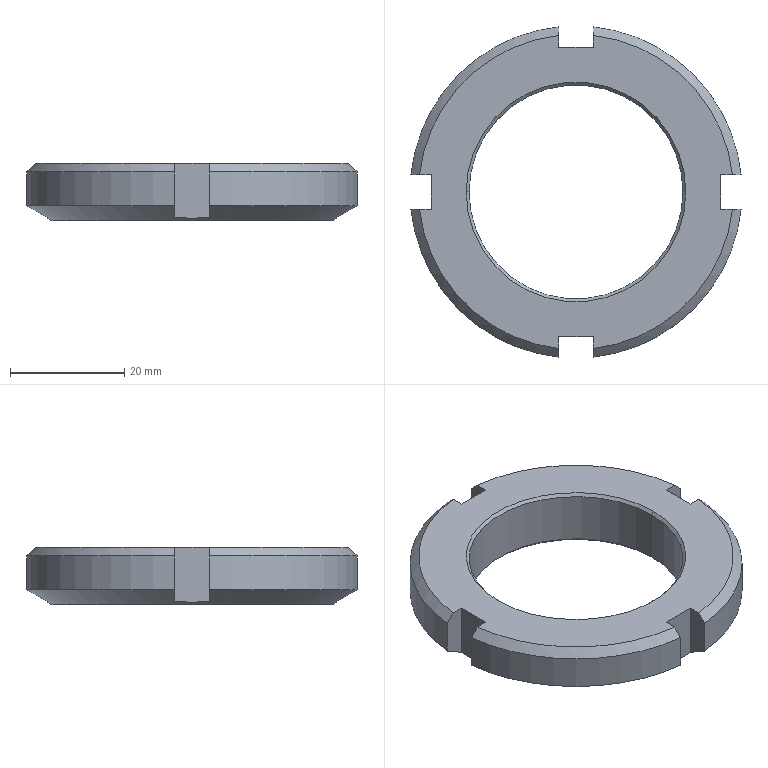Part | SolidWorks | features Chamfer 3, CirPattern 1, Cut 1, Extrusion 1 | 1 solid | 30 faces | box 57.689 x 57.689 x 10 mm | volume 13482 mm3 | plane 14 | cone 10 | cylinder 6 | commonest cylinder face diameters 58 x4 37.376 x2
STEP:
#1=CARTESIAN_POINT('',(-18.688,0.,9.5));
#2=VERTEX_POINT('',#1);
#3=CARTESIAN_POINT('',(18.688,0.,9.5));
#4=VERTEX_POINT('',#3);
#5=CARTESIAN_POINT('',(0.,0.,9.5));
#6=DIRECTION('',(0.,0.,1.));
#7=DIRECTION('',(1.,0.,0.));
#8=AXIS2_PLACEMENT_3D('',#5,#6,#7);
#9=CIRCLE('',#8,18.688);
#10=EDGE_CURVE('',#2,#4,#9,.T.);
#11=ORIENTED_EDGE('',*,*,#10,.F.);
#12=CARTESIAN_POINT('',(-19.188,0.,10.));
#13=VERTEX_POINT('',#12);
#14=CARTESIAN_POINT('',(-18.688,0.,9.5));
#15=DIRECTION('',(-0.7071,0.,0.7071));
#16=VECTOR('',#15,1000.);
#17=LINE('',#14,#16);
#18=EDGE_CURVE('',#2,#13,#17,.T.);
#19=ORIENTED_EDGE('',*,*,#18,.T.);
#20=CARTESIAN_POINT('',(19.188,0.,10.));
#21=VERTEX_POINT('',#20);
#22=CARTESIAN_POINT('',(0.,0.,10.));
#23=DIRECTION('',(0.,0.,-1.));
#24=DIRECTION('',(1.,0.,0.));
#25=AXIS2_PLACEMENT_3D('',#22,#23,#24);
#26=CIRCLE('',#25,19.188);
#27=EDGE_CURVE('',#21,#13,#26,.T.);
#28=ORIENTED_EDGE('',*,*,#27,.F.);
#29=CARTESIAN_POINT('',(18.688,0.,9.5));
#30=DIRECTION('',(0.7071,0.,0.7071));
#31=VECTOR('',#30,1000.);
#32=LINE('',#29,#31);
#33=EDGE_CURVE('',#4,#21,#32,.T.);
#34=ORIENTED_EDGE('',*,*,#33,.F.);
#35=EDGE_LOOP('',(#11,#19,#28,#34));
#36=FACE_OUTER_BOUND('',#35,.T.);
#37=CARTESIAN_POINT('',(0.,0.,9.5));
#38=DIRECTION('',(0.,0.,1.));
#39=DIRECTION('',(1.,0.,0.));
#40=AXIS2_PLACEMENT_3D('',#37,#38,#39);
#41=CONICAL_SURFACE('',#40,18.688,0.7854);
#42=ADVANCED_FACE('',(#36),#41,.F.);
#43=CARTESIAN_POINT('',(18.688,0.,0.5));
#44=VERTEX_POINT('',#43);
#45=CARTESIAN_POINT('',(-18.688,0.,0.5));
#46=VERTEX_POINT('',#45);
#47=CARTESIAN_POINT('',(0.,0.,0.5));
#48=DIRECTION('',(0.,0.,-1.));
#49=DIRECTION('',(1.,0.,0.));
#50=AXIS2_PLACEMENT_3D('',#47,#48,#49);
#51=CIRCLE('',#50,18.688);
#52=EDGE_CURVE('',#44,#46,#51,.T.);
#53=ORIENTED_EDGE('',*,*,#52,.F.);
#54=CARTESIAN_POINT('',(19.188,0.,0.));
#55=VERTEX_POINT('',#54);
#56=CARTESIAN_POINT('',(19.188,0.,0.));
#57=DIRECTION('',(0.7071,0.,-0.7071));
#58=VECTOR('',#57,1000.);
#59=LINE('',#56,#58);
#60=EDGE_CURVE('',#44,#55,#59,.T.);
#61=ORIENTED_EDGE('',*,*,#60,.T.);
#62=CARTESIAN_POINT('',(-19.188,0.,0.));
#63=VERTEX_POINT('',#62);
#64=CARTESIAN_POINT('',(0.,0.,0.));
#65=DIRECTION('',(0.,0.,1.));
#66=DIRECTION('',(1.,0.,0.));
#67=AXIS2_PLACEMENT_3D('',#64,#65,#66);
#68=CIRCLE('',#67,19.188);
#69=EDGE_CURVE('',#63,#55,#68,.T.);
#70=ORIENTED_EDGE('',*,*,#69,.F.);
#71=CARTESIAN_POINT('',(-19.188,0.,0.));
#72=DIRECTION('',(-0.7071,0.,-0.7071));
#73=VECTOR('',#72,1000.);
#74=LINE('',#71,#73);
#75=EDGE_CURVE('',#46,#63,#74,.T.);
#76=ORIENTED_EDGE('',*,*,#75,.F.);
#77=EDGE_LOOP('',(#53,#61,#70,#76));
#78=FACE_OUTER_BOUND('',#77,.T.);
#79=CARTESIAN_POINT('',(0.,0.,0.));
#80=DIRECTION('',(0.,0.,-1.));
#81=DIRECTION('',(-1.,0.,0.));
#82=AXIS2_PLACEMENT_3D('',#79,#80,#81);
#83=CONICAL_SURFACE('',#82,19.188,0.7854);
#84=ADVANCED_FACE('',(#78),#83,.F.);
#85=CARTESIAN_POINT('',(-24.5,0.,0.));
#86=VERTEX_POINT('',#85);
#87=CARTESIAN_POINT('',(24.5,0.,0.));
#88=VERTEX_POINT('',#87);
#89=CARTESIAN_POINT('',(0.,0.,0.));
#90=DIRECTION('',(0.,0.,-1.));
#91=DIRECTION('',(1.,0.,0.));
#92=AXIS2_PLACEMENT_3D('',#89,#90,#91);
#93=CIRCLE('',#92,24.5);
#94=EDGE_CURVE('',#86,#88,#93,.T.);
#95=ORIENTED_EDGE('',*,*,#94,.F.);
#96=CARTESIAN_POINT('',(-25.244,0.,0.4298));
#97=VERTEX_POINT('',#96);
#98=CARTESIAN_POINT('',(-29.,0.,2.598));
#99=DIRECTION('',(-0.866,0.,0.5));
#100=VECTOR('',#99,1000.);
#101=LINE('',#98,#100);
#102=EDGE_CURVE('',#86,#97,#101,.T.);
#103=ORIENTED_EDGE('',*,*,#102,.T.);
#104=CARTESIAN_POINT('',(-25.244,3.,0.5323));
#105=VERTEX_POINT('',#104);
#106=CARTESIAN_POINT('',(-25.244,3.,0.5323));
#107=CARTESIAN_POINT('',(-25.244,2.003,0.4644));
#108=CARTESIAN_POINT('',(-25.244,1.003,0.4298));
#109=CARTESIAN_POINT('',(-25.244,0.,0.4298));
#110=B_SPLINE_CURVE_WITH_KNOTS('',3,(#106,#107,#108,#109),.UNSPECIFIED.,.F.,.F.,(4,4),(0.007992,0.01099),.UNSPECIFIED.);
#111=EDGE_CURVE('',#105,#97,#110,.T.);
#112=ORIENTED_EDGE('',*,*,#111,.F.);
#113=CARTESIAN_POINT('',(-28.844,3.,2.598));
#114=VERTEX_POINT('',#113);
#115=CARTESIAN_POINT('',(-28.844,3.,2.598));
#116=CARTESIAN_POINT('',(-28.638,3.,2.48));
#117=CARTESIAN_POINT('',(-28.432,3.,2.361));
#118=CARTESIAN_POINT('',(-28.226,3.,2.243));
#119=CARTESIAN_POINT('',(-27.232,3.,1.672));
#120=CARTESIAN_POINT('',(-26.238,3.,1.102));
#121=CARTESIAN_POINT('',(-25.244,3.,0.5323));
#122=B_SPLINE_CURVE_WITH_KNOTS('',3,(#115,#116,#117,#118,#119,#120,#121),.UNSPECIFIED.,.F.,.F.,(4,3,4),(0.007772,0.008485,0.01192),.UNSPECIFIED.);
#123=EDGE_CURVE('',#114,#105,#122,.T.);
#124=ORIENTED_EDGE('',*,*,#123,.F.);
#125=CARTESIAN_POINT('',(-3.,28.844,2.598));
#126=VERTEX_POINT('',#125);
#127=CARTESIAN_POINT('',(0.,0.,2.598));
#128=DIRECTION('',(0.,0.,1.));
#129=DIRECTION('',(1.,0.,0.));
#130=AXIS2_PLACEMENT_3D('',#127,#128,#129);
#131=CIRCLE('',#130,29.);
#132=EDGE_CURVE('',#126,#114,#131,.T.);
#133=ORIENTED_EDGE('',*,*,#132,.F.);
#134=CARTESIAN_POINT('',(-3.,25.244,0.5323));
#135=VERTEX_POINT('',#134);
#136=CARTESIAN_POINT('',(-3.,25.244,0.5323));
#137=CARTESIAN_POINT('',(-3.,26.445,1.22));
#138=CARTESIAN_POINT('',(-3.,27.645,1.909));
#139=CARTESIAN_POINT('',(-3.,28.844,2.598));
#140=B_SPLINE_CURVE_WITH_KNOTS('',3,(#136,#137,#138,#139),.UNSPECIFIED.,.F.,.F.,(4,4),(0.008037,0.01219),.UNSPECIFIED.);
#141=EDGE_CURVE('',#135,#126,#140,.T.);
#142=ORIENTED_EDGE('',*,*,#141,.F.);
#143=CARTESIAN_POINT('',(3.,25.244,0.5323));
#144=VERTEX_POINT('',#143);
#145=CARTESIAN_POINT('',(3.,25.244,0.5323));
#146=CARTESIAN_POINT('',(2.006,25.244,0.4646));
#147=CARTESIAN_POINT('',(1.009,25.244,0.43));
#148=CARTESIAN_POINT('',(-0.9914,25.244,0.4296));
#149=CARTESIAN_POINT('',(-1.998,25.244,0.4641));
#150=CARTESIAN_POINT('',(-3.,25.244,0.5323));
#151=B_SPLINE_CURVE_WITH_KNOTS('',3,(#145,#146,#147,#148,#149,#150),.UNSPECIFIED.,.F.,.F.,(4,2,4),(0.007992,0.01098,0.01397),.UNSPECIFIED.);
#152=EDGE_CURVE('',#144,#135,#151,.T.);
#153=ORIENTED_EDGE('',*,*,#152,.F.);
#154=CARTESIAN_POINT('',(3.,28.844,2.598));
#155=VERTEX_POINT('',#154);
#156=CARTESIAN_POINT('',(3.,28.844,2.598));
#157=CARTESIAN_POINT('',(3.,27.645,1.909));
#158=CARTESIAN_POINT('',(3.,26.445,1.22));
#159=CARTESIAN_POINT('',(3.,25.244,0.5323));
#160=B_SPLINE_CURVE_WITH_KNOTS('',3,(#156,#157,#158,#159),.UNSPECIFIED.,.F.,.F.,(4,4),(0.004783,0.008934),.UNSPECIFIED.);
#161=EDGE_CURVE('',#155,#144,#160,.T.);
#162=ORIENTED_EDGE('',*,*,#161,.F.);
#163=CARTESIAN_POINT('',(28.844,3.,2.598));
#164=VERTEX_POINT('',#163);
#165=CARTESIAN_POINT('',(0.,0.,2.598));
#166=DIRECTION('',(0.,0.,1.));
#167=DIRECTION('',(1.,0.,0.));
#168=AXIS2_PLACEMENT_3D('',#165,#166,#167);
#169=CIRCLE('',#168,29.);
#170=EDGE_CURVE('',#164,#155,#169,.T.);
#171=ORIENTED_EDGE('',*,*,#170,.F.);
#172=CARTESIAN_POINT('',(25.244,3.,0.5323));
#173=VERTEX_POINT('',#172);
#174=CARTESIAN_POINT('',(25.244,3.,0.5323));
#175=CARTESIAN_POINT('',(26.445,3.,1.22));
#176=CARTESIAN_POINT('',(27.645,3.,1.909));
#177=CARTESIAN_POINT('',(28.844,3.,2.598));
#178=B_SPLINE_CURVE_WITH_KNOTS('',3,(#174,#175,#176,#177),.UNSPECIFIED.,.F.,.F.,(4,4),(0.008037,0.01219),.UNSPECIFIED.);
#179=EDGE_CURVE('',#173,#164,#178,.T.);
#180=ORIENTED_EDGE('',*,*,#179,.F.);
#181=CARTESIAN_POINT('',(25.244,0.,0.4298));
#182=VERTEX_POINT('',#181);
#183=CARTESIAN_POINT('',(25.244,0.,0.4298));
#184=CARTESIAN_POINT('',(25.244,1.003,0.4298));
#185=CARTESIAN_POINT('',(25.244,2.003,0.4644));
#186=CARTESIAN_POINT('',(25.244,3.,0.5323));
#187=B_SPLINE_CURVE_WITH_KNOTS('',3,(#183,#184,#185,#186),.UNSPECIFIED.,.F.,.F.,(4,4),(0.01545,0.01845),.UNSPECIFIED.);
#188=EDGE_CURVE('',#182,#173,#187,.T.);
#189=ORIENTED_EDGE('',*,*,#188,.F.);
#190=CARTESIAN_POINT('',(29.,0.,2.598));
#191=DIRECTION('',(0.866,0.,0.5));
#192=VECTOR('',#191,1000.);
#193=LINE('',#190,#192);
#194=EDGE_CURVE('',#88,#182,#193,.T.);
#195=ORIENTED_EDGE('',*,*,#194,.F.);
#196=EDGE_LOOP('',(#95,#103,#112,#124,#133,#142,#153,#162,#171,#180,#189,#195));
#197=FACE_OUTER_BOUND('',#196,.T.);
#198=CARTESIAN_POINT('',(0.,0.,2.598));
#199=DIRECTION('',(0.,0.,1.));
#200=DIRECTION('',(1.,0.,0.));
#201=AXIS2_PLACEMENT_3D('',#198,#199,#200);
#202=CONICAL_SURFACE('',#201,29.,1.047);
#203=ADVANCED_FACE('',(#197),#202,.T.);
#204=ORIENTED_EDGE('',*,*,#10,.T.);
#205=CARTESIAN_POINT('',(18.688,0.,10.));
#206=DIRECTION('',(0.,0.,-1.));
#207=VECTOR('',#206,1000.);
#208=LINE('',#205,#207);
#209=EDGE_CURVE('',#4,#44,#208,.T.);
#210=ORIENTED_EDGE('',*,*,#209,.T.);
#211=ORIENTED_EDGE('',*,*,#52,.T.);
#212=CARTESIAN_POINT('',(-18.688,0.,10.));
#213=DIRECTION('',(0.,0.,-1.));
#214=VECTOR('',#213,1000.);
#215=LINE('',#212,#214);
#216=EDGE_CURVE('',#2,#46,#215,.T.);
#217=ORIENTED_EDGE('',*,*,#216,.F.);
#218=EDGE_LOOP('',(#204,#210,#211,#217));
#219=FACE_OUTER_BOUND('',#218,.T.);
#220=CARTESIAN_POINT('',(0.,0.,10.));
#221=DIRECTION('',(0.,0.,-1.));
#222=DIRECTION('',(-1.,0.,0.));
#223=AXIS2_PLACEMENT_3D('',#220,#221,#222);
#224=CYLINDRICAL_SURFACE('',#223,18.688);
#225=ADVANCED_FACE('',(#219),#224,.F.);
#226=CARTESIAN_POINT('',(3.,28.844,8.5));
#227=VERTEX_POINT('',#226);
#228=CARTESIAN_POINT('',(28.844,3.,8.5));
#229=VERTEX_POINT('',#228);
#230=CARTESIAN_POINT('',(0.,0.,8.5));
#231=DIRECTION('',(0.,0.,-1.));
#232=DIRECTION('',(1.,0.,0.));
#233=AXIS2_PLACEMENT_3D('',#230,#231,#232);
#234=CIRCLE('',#233,29.);
#235=EDGE_CURVE('',#227,#229,#234,.T.);
#236=ORIENTED_EDGE('',*,*,#235,.T.);
#237=CARTESIAN_POINT('',(28.844,3.,0.));
#238=DIRECTION('',(0.,0.,1.));
#239=VECTOR('',#238,1000.);
#240=LINE('',#237,#239);
#241=EDGE_CURVE('',#164,#229,#240,.T.);
#242=ORIENTED_EDGE('',*,*,#241,.F.);
#243=ORIENTED_EDGE('',*,*,#170,.T.);
#244=CARTESIAN_POINT('',(3.,28.844,0.));
#245=DIRECTION('',(0.,0.,1.));
#246=VECTOR('',#245,1000.);
#247=LINE('',#244,#246);
#248=EDGE_CURVE('',#155,#227,#247,.T.);
#249=ORIENTED_EDGE('',*,*,#248,.T.);
#250=EDGE_LOOP('',(#236,#242,#243,#249));
#251=FACE_OUTER_BOUND('',#250,.T.);
#252=CARTESIAN_POINT('',(0.,0.,10.));
#253=DIRECTION('',(0.,0.,-1.));
#254=DIRECTION('',(-1.,0.,0.));
#255=AXIS2_PLACEMENT_3D('',#252,#253,#254);
#256=CYLINDRICAL_SURFACE('',#255,29.);
#257=ADVANCED_FACE('',(#251),#256,.T.);
#258=CARTESIAN_POINT('',(27.336,3.,10.));
#259=VERTEX_POINT('',#258);
#260=CARTESIAN_POINT('',(28.844,3.,8.5));
#261=CARTESIAN_POINT('',(28.431,3.,8.911));
#262=CARTESIAN_POINT('',(28.017,3.,9.323));
#263=CARTESIAN_POINT('',(27.603,3.,9.734));
#264=CARTESIAN_POINT('',(27.514,3.,9.823));
#265=CARTESIAN_POINT('',(27.425,3.,9.911));
#266=CARTESIAN_POINT('',(27.336,3.,10.));
#267=B_SPLINE_CURVE_WITH_KNOTS('',3,(#260,#261,#262,#263,#264,#265,#266),.UNSPECIFIED.,.F.,.F.,(4,3,4),(0.006071,0.007821,0.008198),.UNSPECIFIED.);
#268=EDGE_CURVE('',#229,#259,#267,.T.);
#269=ORIENTED_EDGE('',*,*,#268,.F.);
#270=ORIENTED_EDGE('',*,*,#235,.F.);
#271=CARTESIAN_POINT('',(3.,27.336,10.));
#272=VERTEX_POINT('',#271);
#273=CARTESIAN_POINT('',(3.,27.336,10.));
#274=CARTESIAN_POINT('',(3.,27.425,9.911));
#275=CARTESIAN_POINT('',(3.,27.514,9.823));
#276=CARTESIAN_POINT('',(3.,27.603,9.734));
#277=CARTESIAN_POINT('',(3.,28.017,9.323));
#278=CARTESIAN_POINT('',(3.,28.431,8.911));
#279=CARTESIAN_POINT('',(3.,28.844,8.5));
#280=B_SPLINE_CURVE_WITH_KNOTS('',3,(#273,#274,#275,#276,#277,#278,#279),.UNSPECIFIED.,.F.,.F.,(4,3,4),(0.007445,0.007821,0.009572),.UNSPECIFIED.);
#281=EDGE_CURVE('',#272,#227,#280,.T.);
#282=ORIENTED_EDGE('',*,*,#281,.F.);
#283=CARTESIAN_POINT('',(0.,0.,10.));
#284=DIRECTION('',(0.,0.,1.));
#285=DIRECTION('',(1.,0.,0.));
#286=AXIS2_PLACEMENT_3D('',#283,#284,#285);
#287=CIRCLE('',#286,27.5);
#288=EDGE_CURVE('',#259,#272,#287,.T.);
#289=ORIENTED_EDGE('',*,*,#288,.F.);
#290=EDGE_LOOP('',(#269,#270,#282,#289));
#291=FACE_OUTER_BOUND('',#290,.T.);
#292=CARTESIAN_POINT('',(0.,0.,10.));
#293=DIRECTION('',(0.,0.,-1.));
#294=DIRECTION('',(-1.,0.,0.));
#295=AXIS2_PLACEMENT_3D('',#292,#293,#294);
#296=CONICAL_SURFACE('',#295,27.5,0.7854);
#297=ADVANCED_FACE('',(#291),#296,.T.);
#298=CARTESIAN_POINT('',(-28.844,3.,8.5));
#299=VERTEX_POINT('',#298);
#300=CARTESIAN_POINT('',(-3.,28.844,8.5));
#301=VERTEX_POINT('',#300);
#302=CARTESIAN_POINT('',(0.,0.,8.5));
#303=DIRECTION('',(0.,0.,-1.));
#304=DIRECTION('',(1.,0.,0.));
#305=AXIS2_PLACEMENT_3D('',#302,#303,#304);
#306=CIRCLE('',#305,29.);
#307=EDGE_CURVE('',#299,#301,#306,.T.);
#308=ORIENTED_EDGE('',*,*,#307,.T.);
#309=CARTESIAN_POINT('',(-3.,28.844,0.));
#310=DIRECTION('',(0.,0.,1.));
#311=VECTOR('',#310,1000.);
#312=LINE('',#309,#311);
#313=EDGE_CURVE('',#126,#301,#312,.T.);
#314=ORIENTED_EDGE('',*,*,#313,.F.);
#315=ORIENTED_EDGE('',*,*,#132,.T.);
#316=CARTESIAN_POINT('',(-28.844,3.,0.));
#317=DIRECTION('',(0.,0.,1.));
#318=VECTOR('',#317,1000.);
#319=LINE('',#316,#318);
#320=EDGE_CURVE('',#114,#299,#319,.T.);
#321=ORIENTED_EDGE('',*,*,#320,.T.);
#322=EDGE_LOOP('',(#308,#314,#315,#321));
#323=FACE_OUTER_BOUND('',#322,.T.);
#324=CARTESIAN_POINT('',(0.,0.,10.));
#325=DIRECTION('',(0.,0.,-1.));
#326=DIRECTION('',(-1.,0.,0.));
#327=AXIS2_PLACEMENT_3D('',#324,#325,#326);
#328=CYLINDRICAL_SURFACE('',#327,29.);
#329=ADVANCED_FACE('',(#323),#328,.T.);
#330=CARTESIAN_POINT('',(-3.,27.336,10.));
#331=VERTEX_POINT('',#330);
#332=CARTESIAN_POINT('',(-3.,28.844,8.5));
#333=CARTESIAN_POINT('',(-3.,28.431,8.911));
#334=CARTESIAN_POINT('',(-3.,28.017,9.323));
#335=CARTESIAN_POINT('',(-3.,27.603,9.734));
#336=CARTESIAN_POINT('',(-3.,27.514,9.823));
#337=CARTESIAN_POINT('',(-3.,27.425,9.911));
#338=CARTESIAN_POINT('',(-3.,27.336,10.));
#339=B_SPLINE_CURVE_WITH_KNOTS('',3,(#332,#333,#334,#335,#336,#337,#338),.UNSPECIFIED.,.F.,.F.,(4,3,4),(0.006071,0.007821,0.008198),.UNSPECIFIED.);
#340=EDGE_CURVE('',#301,#331,#339,.T.);
#341=ORIENTED_EDGE('',*,*,#340,.F.);
#342=ORIENTED_EDGE('',*,*,#307,.F.);
#343=CARTESIAN_POINT('',(-27.336,3.,10.));
#344=VERTEX_POINT('',#343);
#345=CARTESIAN_POINT('',(-27.336,3.,10.));
#346=CARTESIAN_POINT('',(-27.701,3.,9.637));
#347=CARTESIAN_POINT('',(-28.066,3.,9.274));
#348=CARTESIAN_POINT('',(-28.431,3.,8.911));
#349=CARTESIAN_POINT('',(-28.569,3.,8.774));
#350=CARTESIAN_POINT('',(-28.707,3.,8.637));
#351=CARTESIAN_POINT('',(-28.844,3.,8.5));
#352=B_SPLINE_CURVE_WITH_KNOTS('',3,(#345,#346,#347,#348,#349,#350,#351),.UNSPECIFIED.,.F.,.F.,(4,3,4),(0.006278,0.007821,0.008405),.UNSPECIFIED.);
#353=EDGE_CURVE('',#344,#299,#352,.T.);
#354=ORIENTED_EDGE('',*,*,#353,.F.);
#355=CARTESIAN_POINT('',(0.,0.,10.));
#356=DIRECTION('',(0.,0.,1.));
#357=DIRECTION('',(1.,0.,0.));
#358=AXIS2_PLACEMENT_3D('',#355,#356,#357);
#359=CIRCLE('',#358,27.5);
#360=EDGE_CURVE('',#331,#344,#359,.T.);
#361=ORIENTED_EDGE('',*,*,#360,.F.);
#362=EDGE_LOOP('',(#341,#342,#354,#361));
#363=FACE_OUTER_BOUND('',#362,.T.);
#364=CARTESIAN_POINT('',(0.,0.,10.));
#365=DIRECTION('',(0.,0.,-1.));
#366=DIRECTION('',(-1.,0.,0.));
#367=AXIS2_PLACEMENT_3D('',#364,#365,#366);
#368=CONICAL_SURFACE('',#367,27.5,0.7854);
#369=ADVANCED_FACE('',(#363),#368,.T.);
#370=CARTESIAN_POINT('',(-3.,-28.844,8.5));
#371=VERTEX_POINT('',#370);
#372=CARTESIAN_POINT('',(-28.844,-3.,8.5));
#373=VERTEX_POINT('',#372);
#374=CARTESIAN_POINT('',(0.,0.,8.5));
#375=DIRECTION('',(0.,0.,-1.));
#376=DIRECTION('',(1.,0.,0.));
#377=AXIS2_PLACEMENT_3D('',#374,#375,#376);
#378=CIRCLE('',#377,29.);
#379=EDGE_CURVE('',#371,#373,#378,.T.);
#380=ORIENTED_EDGE('',*,*,#379,.T.);
#381=CARTESIAN_POINT('',(-28.844,-3.,2.598));
#382=VERTEX_POINT('',#381);
#383=CARTESIAN_POINT('',(-28.844,-3.,0.));
#384=DIRECTION('',(0.,0.,1.));
#385=VECTOR('',#384,1000.);
#386=LINE('',#383,#385);
#387=EDGE_CURVE('',#382,#373,#386,.T.);
#388=ORIENTED_EDGE('',*,*,#387,.F.);
#389=CARTESIAN_POINT('',(-3.,-28.844,2.598));
#390=VERTEX_POINT('',#389);
#391=CARTESIAN_POINT('',(0.,0.,2.598));
#392=DIRECTION('',(0.,0.,1.));
#393=DIRECTION('',(1.,0.,0.));
#394=AXIS2_PLACEMENT_3D('',#391,#392,#393);
#395=CIRCLE('',#394,29.);
#396=EDGE_CURVE('',#382,#390,#395,.T.);
#397=ORIENTED_EDGE('',*,*,#396,.T.);
#398=CARTESIAN_POINT('',(-3.,-28.844,0.));
#399=DIRECTION('',(0.,0.,1.));
#400=VECTOR('',#399,1000.);
#401=LINE('',#398,#400);
#402=EDGE_CURVE('',#390,#371,#401,.T.);
#403=ORIENTED_EDGE('',*,*,#402,.T.);
#404=EDGE_LOOP('',(#380,#388,#397,#403));
#405=FACE_OUTER_BOUND('',#404,.T.);
#406=CARTESIAN_POINT('',(0.,0.,10.));
#407=DIRECTION('',(0.,0.,-1.));
#408=DIRECTION('',(-1.,0.,0.));
#409=AXIS2_PLACEMENT_3D('',#406,#407,#408);
#410=CYLINDRICAL_SURFACE('',#409,29.);
#411=ADVANCED_FACE('',(#405),#410,.T.);
#412=CARTESIAN_POINT('',(-27.336,-3.,10.));
#413=VERTEX_POINT('',#412);
#414=CARTESIAN_POINT('',(-28.844,-3.,8.5));
#415=CARTESIAN_POINT('',(-28.707,-3.,8.637));
#416=CARTESIAN_POINT('',(-28.569,-3.,8.774));
#417=CARTESIAN_POINT('',(-28.431,-3.,8.911));
#418=CARTESIAN_POINT('',(-28.066,-3.,9.274));
#419=CARTESIAN_POINT('',(-27.701,-3.,9.637));
#420=CARTESIAN_POINT('',(-27.336,-3.,10.));
#421=B_SPLINE_CURVE_WITH_KNOTS('',3,(#414,#415,#416,#417,#418,#419,#420),.UNSPECIFIED.,.F.,.F.,(4,3,4),(0.007238,0.007821,0.009365),.UNSPECIFIED.);
#422=EDGE_CURVE('',#373,#413,#421,.T.);
#423=ORIENTED_EDGE('',*,*,#422,.F.);
#424=ORIENTED_EDGE('',*,*,#379,.F.);
#425=CARTESIAN_POINT('',(-3.,-27.336,10.));
#426=VERTEX_POINT('',#425);
#427=CARTESIAN_POINT('',(-3.,-27.336,10.));
#428=CARTESIAN_POINT('',(-3.,-27.701,9.637));
#429=CARTESIAN_POINT('',(-3.,-28.066,9.274));
#430=CARTESIAN_POINT('',(-3.,-28.431,8.911));
#431=CARTESIAN_POINT('',(-3.,-28.569,8.774));
#432=CARTESIAN_POINT('',(-3.,-28.707,8.637));
#433=CARTESIAN_POINT('',(-3.,-28.844,8.5));
#434=B_SPLINE_CURVE_WITH_KNOTS('',3,(#427,#428,#429,#430,#431,#432,#433),.UNSPECIFIED.,.F.,.F.,(4,3,4),(0.006278,0.007821,0.008405),.UNSPECIFIED.);
#435=EDGE_CURVE('',#426,#371,#434,.T.);
#436=ORIENTED_EDGE('',*,*,#435,.F.);
#437=CARTESIAN_POINT('',(0.,0.,10.));
#438=DIRECTION('',(0.,0.,1.));
#439=DIRECTION('',(1.,0.,0.));
#440=AXIS2_PLACEMENT_3D('',#437,#438,#439);
#441=CIRCLE('',#440,27.5);
#442=EDGE_CURVE('',#413,#426,#441,.T.);
#443=ORIENTED_EDGE('',*,*,#442,.F.);
#444=EDGE_LOOP('',(#423,#424,#436,#443));
#445=FACE_OUTER_BOUND('',#444,.T.);
#446=CARTESIAN_POINT('',(0.,0.,10.));
#447=DIRECTION('',(0.,0.,-1.));
#448=DIRECTION('',(-1.,0.,0.));
#449=AXIS2_PLACEMENT_3D('',#446,#447,#448);
#450=CONICAL_SURFACE('',#449,27.5,0.7854);
#451=ADVANCED_FACE('',(#445),#450,.T.);
#452=ORIENTED_EDGE('',*,*,#27,.T.);
#453=CARTESIAN_POINT('',(0.,0.,10.));
#454=DIRECTION('',(0.,0.,-1.));
#455=DIRECTION('',(1.,0.,0.));
#456=AXIS2_PLACEMENT_3D('',#453,#454,#455);
#457=CIRCLE('',#456,19.188);
#458=EDGE_CURVE('',#13,#21,#457,.T.);
#459=ORIENTED_EDGE('',*,*,#458,.T.);
#460=EDGE_LOOP('',(#452,#459));
#461=FACE_BOUND('',#460,.T.);
#462=CARTESIAN_POINT('',(25.244,3.,10.));
#463=VERTEX_POINT('',#462);
#464=CARTESIAN_POINT('',(25.244,3.,10.));
#465=DIRECTION('',(-1.,0.,0.));
#466=VECTOR('',#465,1000.);
#467=LINE('',#464,#466);
#468=EDGE_CURVE('',#259,#463,#467,.T.);
#469=ORIENTED_EDGE('',*,*,#468,.F.);
#470=ORIENTED_EDGE('',*,*,#288,.T.);
#471=CARTESIAN_POINT('',(3.,25.244,10.));
#472=VERTEX_POINT('',#471);
#473=CARTESIAN_POINT('',(3.,25.244,10.));
#474=DIRECTION('',(0.,1.,0.));
#475=VECTOR('',#474,1000.);
#476=LINE('',#473,#475);
#477=EDGE_CURVE('',#472,#272,#476,.T.);
#478=ORIENTED_EDGE('',*,*,#477,.F.);
#479=CARTESIAN_POINT('',(-3.,25.244,10.));
#480=VERTEX_POINT('',#479);
#481=CARTESIAN_POINT('',(3.,25.244,10.));
#482=DIRECTION('',(1.,0.,0.));
#483=VECTOR('',#482,1000.);
#484=LINE('',#481,#483);
#485=EDGE_CURVE('',#480,#472,#484,.T.);
#486=ORIENTED_EDGE('',*,*,#485,.F.);
#487=CARTESIAN_POINT('',(-3.,25.244,10.));
#488=DIRECTION('',(0.,-1.,0.));
#489=VECTOR('',#488,1000.);
#490=LINE('',#487,#489);
#491=EDGE_CURVE('',#331,#480,#490,.T.);
#492=ORIENTED_EDGE('',*,*,#491,.F.);
#493=ORIENTED_EDGE('',*,*,#360,.T.);
#494=CARTESIAN_POINT('',(-25.244,3.,10.));
#495=VERTEX_POINT('',#494);
#496=CARTESIAN_POINT('',(-25.244,3.,10.));
#497=DIRECTION('',(-1.,0.,0.));
#498=VECTOR('',#497,1000.);
#499=LINE('',#496,#498);
#500=EDGE_CURVE('',#495,#344,#499,.T.);
#501=ORIENTED_EDGE('',*,*,#500,.F.);
#502=CARTESIAN_POINT('',(-25.244,-3.,10.));
#503=VERTEX_POINT('',#502);
#504=CARTESIAN_POINT('',(-25.244,3.,10.));
#505=DIRECTION('',(0.,1.,0.));
#506=VECTOR('',#505,1000.);
#507=LINE('',#504,#506);
#508=EDGE_CURVE('',#503,#495,#507,.T.);
#509=ORIENTED_EDGE('',*,*,#508,.F.);
#510=CARTESIAN_POINT('',(-25.244,-3.,10.));
#511=DIRECTION('',(1.,0.,0.));
#512=VECTOR('',#511,1000.);
#513=LINE('',#510,#512);
#514=EDGE_CURVE('',#413,#503,#513,.T.);
#515=ORIENTED_EDGE('',*,*,#514,.F.);
#516=ORIENTED_EDGE('',*,*,#442,.T.);
#517=CARTESIAN_POINT('',(-3.,-25.244,10.));
#518=VERTEX_POINT('',#517);
#519=CARTESIAN_POINT('',(-3.,-25.244,10.));
#520=DIRECTION('',(0.,-1.,0.));
#521=VECTOR('',#520,1000.);
#522=LINE('',#519,#521);
#523=EDGE_CURVE('',#518,#426,#522,.T.);
#524=ORIENTED_EDGE('',*,*,#523,.F.);
#525=CARTESIAN_POINT('',(3.,-25.244,10.));
#526=VERTEX_POINT('',#525);
#527=CARTESIAN_POINT('',(-3.,-25.244,10.));
#528=DIRECTION('',(-1.,0.,0.));
#529=VECTOR('',#528,1000.);
#530=LINE('',#527,#529);
#531=EDGE_CURVE('',#526,#518,#530,.T.);
#532=ORIENTED_EDGE('',*,*,#531,.F.);
#533=CARTESIAN_POINT('',(3.,-27.336,10.));
#534=VERTEX_POINT('',#533);
#535=CARTESIAN_POINT('',(3.,-25.244,10.));
#536=DIRECTION('',(0.,1.,0.));
#537=VECTOR('',#536,1000.);
#538=LINE('',#535,#537);
#539=EDGE_CURVE('',#534,#526,#538,.T.);
#540=ORIENTED_EDGE('',*,*,#539,.F.);
#541=CARTESIAN_POINT('',(27.336,-3.,10.));
#542=VERTEX_POINT('',#541);
#543=CARTESIAN_POINT('',(0.,0.,10.));
#544=DIRECTION('',(0.,0.,1.));
#545=DIRECTION('',(1.,0.,0.));
#546=AXIS2_PLACEMENT_3D('',#543,#544,#545);
#547=CIRCLE('',#546,27.5);
#548=EDGE_CURVE('',#534,#542,#547,.T.);
#549=ORIENTED_EDGE('',*,*,#548,.T.);
#550=CARTESIAN_POINT('',(25.244,-3.,10.));
#551=VERTEX_POINT('',#550);
#552=CARTESIAN_POINT('',(25.244,-3.,10.));
#553=DIRECTION('',(1.,0.,0.));
#554=VECTOR('',#553,1000.);
#555=LINE('',#552,#554);
#556=EDGE_CURVE('',#551,#542,#555,.T.);
#557=ORIENTED_EDGE('',*,*,#556,.F.);
#558=CARTESIAN_POINT('',(25.244,-3.,10.));
#559=DIRECTION('',(0.,-1.,0.));
#560=VECTOR('',#559,1000.);
#561=LINE('',#558,#560);
#562=EDGE_CURVE('',#463,#551,#561,.T.);
#563=ORIENTED_EDGE('',*,*,#562,.F.);
#564=EDGE_LOOP('',(#469,#470,#478,#486,#492,#493,#501,#509,#515,#516,#524,#532,#540,#549,#557,#563));
#565=FACE_OUTER_BOUND('',#564,.T.);
#566=CARTESIAN_POINT('',(0.,0.,10.));
#567=DIRECTION('',(0.,0.,1.));
#568=DIRECTION('',(1.,0.,0.));
#569=AXIS2_PLACEMENT_3D('',#566,#567,#568);
#570=PLANE('',#569);
#571=ADVANCED_FACE('',(#461,#565),#570,.T.);
#572=ORIENTED_EDGE('',*,*,#69,.T.);
#573=CARTESIAN_POINT('',(0.,0.,0.));
#574=DIRECTION('',(0.,0.,1.));
#575=DIRECTION('',(1.,0.,0.));
#576=AXIS2_PLACEMENT_3D('',#573,#574,#575);
#577=CIRCLE('',#576,19.188);
#578=EDGE_CURVE('',#55,#63,#577,.T.);
#579=ORIENTED_EDGE('',*,*,#578,.T.);
#580=EDGE_LOOP('',(#572,#579));
#581=FACE_BOUND('',#580,.T.);
#582=CARTESIAN_POINT('',(0.,0.,0.));
#583=DIRECTION('',(0.,0.,-1.));
#584=DIRECTION('',(1.,0.,0.));
#585=AXIS2_PLACEMENT_3D('',#582,#583,#584);
#586=CIRCLE('',#585,24.5);
#587=EDGE_CURVE('',#88,#86,#586,.T.);
#588=ORIENTED_EDGE('',*,*,#587,.T.);
#589=ORIENTED_EDGE('',*,*,#94,.T.);
#590=EDGE_LOOP('',(#588,#589));
#591=FACE_OUTER_BOUND('',#590,.T.);
#592=CARTESIAN_POINT('',(0.,0.,0.));
#593=DIRECTION('',(0.,0.,1.));
#594=DIRECTION('',(1.,0.,0.));
#595=AXIS2_PLACEMENT_3D('',#592,#593,#594);
#596=PLANE('',#595);
#597=ADVANCED_FACE('',(#581,#591),#596,.F.);
#598=CARTESIAN_POINT('',(3.,-28.844,2.598));
#599=VERTEX_POINT('',#598);
#600=CARTESIAN_POINT('',(28.844,-3.,2.598));
#601=VERTEX_POINT('',#600);
#602=CARTESIAN_POINT('',(0.,0.,2.598));
#603=DIRECTION('',(0.,0.,1.));
#604=DIRECTION('',(1.,0.,0.));
#605=AXIS2_PLACEMENT_3D('',#602,#603,#604);
#606=CIRCLE('',#605,29.);
#607=EDGE_CURVE('',#599,#601,#606,.T.);
#608=ORIENTED_EDGE('',*,*,#607,.T.);
#609=CARTESIAN_POINT('',(28.844,-3.,8.5));
#610=VERTEX_POINT('',#609);
#611=CARTESIAN_POINT('',(28.844,-3.,0.));
#612=DIRECTION('',(0.,0.,1.));
#613=VECTOR('',#612,1000.);
#614=LINE('',#611,#613);
#615=EDGE_CURVE('',#601,#610,#614,.T.);
#616=ORIENTED_EDGE('',*,*,#615,.T.);
#617=CARTESIAN_POINT('',(3.,-28.844,8.5));
#618=VERTEX_POINT('',#617);
#619=CARTESIAN_POINT('',(0.,0.,8.5));
#620=DIRECTION('',(0.,0.,-1.));
#621=DIRECTION('',(1.,0.,0.));
#622=AXIS2_PLACEMENT_3D('',#619,#620,#621);
#623=CIRCLE('',#622,29.);
#624=EDGE_CURVE('',#610,#618,#623,.T.);
#625=ORIENTED_EDGE('',*,*,#624,.T.);
#626=CARTESIAN_POINT('',(3.,-28.844,0.));
#627=DIRECTION('',(0.,0.,1.));
#628=VECTOR('',#627,1000.);
#629=LINE('',#626,#628);
#630=EDGE_CURVE('',#599,#618,#629,.T.);
#631=ORIENTED_EDGE('',*,*,#630,.F.);
#632=EDGE_LOOP('',(#608,#616,#625,#631));
#633=FACE_OUTER_BOUND('',#632,.T.);
#634=CARTESIAN_POINT('',(0.,0.,10.));
#635=DIRECTION('',(0.,0.,-1.));
#636=DIRECTION('',(-1.,0.,0.));
#637=AXIS2_PLACEMENT_3D('',#634,#635,#636);
#638=CYLINDRICAL_SURFACE('',#637,29.);
#639=ADVANCED_FACE('',(#633),#638,.T.);
#640=ORIENTED_EDGE('',*,*,#209,.F.);
#641=CARTESIAN_POINT('',(0.,0.,9.5));
#642=DIRECTION('',(0.,0.,1.));
#643=DIRECTION('',(1.,0.,0.));
#644=AXIS2_PLACEMENT_3D('',#641,#642,#643);
#645=CIRCLE('',#644,18.688);
#646=EDGE_CURVE('',#4,#2,#645,.T.);
#647=ORIENTED_EDGE('',*,*,#646,.T.);
#648=ORIENTED_EDGE('',*,*,#216,.T.);
#649=CARTESIAN_POINT('',(0.,0.,0.5));
#650=DIRECTION('',(0.,0.,-1.));
#651=DIRECTION('',(1.,0.,0.));
#652=AXIS2_PLACEMENT_3D('',#649,#650,#651);
#653=CIRCLE('',#652,18.688);
#654=EDGE_CURVE('',#46,#44,#653,.T.);
#655=ORIENTED_EDGE('',*,*,#654,.T.);
#656=EDGE_LOOP('',(#640,#647,#648,#655));
#657=FACE_OUTER_BOUND('',#656,.T.);
#658=CARTESIAN_POINT('',(0.,0.,10.));
#659=DIRECTION('',(0.,0.,-1.));
#660=DIRECTION('',(-1.,0.,0.));
#661=AXIS2_PLACEMENT_3D('',#658,#659,#660);
#662=CYLINDRICAL_SURFACE('',#661,18.688);
#663=ADVANCED_FACE('',(#657),#662,.F.);
#664=CARTESIAN_POINT('',(27.336,-3.,10.));
#665=CARTESIAN_POINT('',(27.425,-3.,9.911));
#666=CARTESIAN_POINT('',(27.514,-3.,9.823));
#667=CARTESIAN_POINT('',(27.603,-3.,9.734));
#668=CARTESIAN_POINT('',(28.017,-3.,9.323));
#669=CARTESIAN_POINT('',(28.431,-3.,8.911));
#670=CARTESIAN_POINT('',(28.844,-3.,8.5));
#671=B_SPLINE_CURVE_WITH_KNOTS('',3,(#664,#665,#666,#667,#668,#669,#670),.UNSPECIFIED.,.F.,.F.,(4,3,4),(0.007445,0.007821,0.009572),.UNSPECIFIED.);
#672=EDGE_CURVE('',#542,#610,#671,.T.);
#673=ORIENTED_EDGE('',*,*,#672,.F.);
#674=ORIENTED_EDGE('',*,*,#548,.F.);
#675=CARTESIAN_POINT('',(3.,-28.844,8.5));
#676=CARTESIAN_POINT('',(3.,-28.707,8.637));
#677=CARTESIAN_POINT('',(3.,-28.569,8.774));
#678=CARTESIAN_POINT('',(3.,-28.431,8.911));
#679=CARTESIAN_POINT('',(3.,-28.066,9.274));
#680=CARTESIAN_POINT('',(3.,-27.701,9.637));
#681=CARTESIAN_POINT('',(3.,-27.336,10.));
#682=B_SPLINE_CURVE_WITH_KNOTS('',3,(#675,#676,#677,#678,#679,#680,#681),.UNSPECIFIED.,.F.,.F.,(4,3,4),(0.007238,0.007821,0.009365),.UNSPECIFIED.);
#683=EDGE_CURVE('',#618,#534,#682,.T.);
#684=ORIENTED_EDGE('',*,*,#683,.F.);
#685=ORIENTED_EDGE('',*,*,#624,.F.);
#686=EDGE_LOOP('',(#673,#674,#684,#685));
#687=FACE_OUTER_BOUND('',#686,.T.);
#688=CARTESIAN_POINT('',(0.,0.,10.));
#689=DIRECTION('',(0.,0.,-1.));
#690=DIRECTION('',(-1.,0.,0.));
#691=AXIS2_PLACEMENT_3D('',#688,#689,#690);
#692=CONICAL_SURFACE('',#691,27.5,0.7854);
#693=ADVANCED_FACE('',(#687),#692,.T.);
#694=ORIENTED_EDGE('',*,*,#102,.F.);
#695=ORIENTED_EDGE('',*,*,#587,.F.);
#696=ORIENTED_EDGE('',*,*,#194,.T.);
#697=CARTESIAN_POINT('',(25.244,-3.,0.5323));
#698=VERTEX_POINT('',#697);
#699=CARTESIAN_POINT('',(25.244,-3.,0.5323));
#700=CARTESIAN_POINT('',(25.244,-2.001,0.4643));
#701=CARTESIAN_POINT('',(25.244,-0.9973,0.4298));
#702=CARTESIAN_POINT('',(25.244,0.,0.4298));
#703=B_SPLINE_CURVE_WITH_KNOTS('',3,(#699,#700,#701,#702),.UNSPECIFIED.,.F.,.F.,(4,4),(0.01247,0.01545),.UNSPECIFIED.);
#704=EDGE_CURVE('',#698,#182,#703,.T.);
#705=ORIENTED_EDGE('',*,*,#704,.F.);
#706=CARTESIAN_POINT('',(28.844,-3.,2.598));
#707=CARTESIAN_POINT('',(27.645,-3.,1.909));
#708=CARTESIAN_POINT('',(26.445,-3.,1.22));
#709=CARTESIAN_POINT('',(25.244,-3.,0.5323));
#710=B_SPLINE_CURVE_WITH_KNOTS('',3,(#706,#707,#708,#709),.UNSPECIFIED.,.F.,.F.,(4,4),(0.004783,0.008934),.UNSPECIFIED.);
#711=EDGE_CURVE('',#601,#698,#710,.T.);
#712=ORIENTED_EDGE('',*,*,#711,.F.);
#713=ORIENTED_EDGE('',*,*,#607,.F.);
#714=CARTESIAN_POINT('',(3.,-25.244,0.5323));
#715=VERTEX_POINT('',#714);
#716=CARTESIAN_POINT('',(3.,-25.244,0.5323));
#717=CARTESIAN_POINT('',(3.,-26.238,1.102));
#718=CARTESIAN_POINT('',(3.,-27.232,1.672));
#719=CARTESIAN_POINT('',(3.,-28.226,2.243));
#720=CARTESIAN_POINT('',(3.,-28.432,2.361));
#721=CARTESIAN_POINT('',(3.,-28.638,2.48));
#722=CARTESIAN_POINT('',(3.,-28.844,2.598));
#723=B_SPLINE_CURVE_WITH_KNOTS('',3,(#716,#717,#718,#719,#720,#721,#722),.UNSPECIFIED.,.F.,.F.,(4,3,4),(0.005048,0.008485,0.009199),.UNSPECIFIED.);
#724=EDGE_CURVE('',#715,#599,#723,.T.);
#725=ORIENTED_EDGE('',*,*,#724,.F.);
#726=CARTESIAN_POINT('',(-3.,-25.244,0.5323));
#727=VERTEX_POINT('',#726);
#728=CARTESIAN_POINT('',(-3.,-25.244,0.5323));
#729=CARTESIAN_POINT('',(-1.998,-25.244,0.4641));
#730=CARTESIAN_POINT('',(-0.9914,-25.244,0.4296));
#731=CARTESIAN_POINT('',(1.009,-25.244,0.43));
#732=CARTESIAN_POINT('',(2.006,-25.244,0.4646));
#733=CARTESIAN_POINT('',(3.,-25.244,0.5323));
#734=B_SPLINE_CURVE_WITH_KNOTS('',3,(#728,#729,#730,#731,#732,#733),.UNSPECIFIED.,.F.,.F.,(4,2,4),(0.01247,0.01546,0.01845),.UNSPECIFIED.);
#735=EDGE_CURVE('',#727,#715,#734,.T.);
#736=ORIENTED_EDGE('',*,*,#735,.F.);
#737=CARTESIAN_POINT('',(-3.,-28.844,2.598));
#738=CARTESIAN_POINT('',(-3.,-28.638,2.48));
#739=CARTESIAN_POINT('',(-3.,-28.432,2.361));
#740=CARTESIAN_POINT('',(-3.,-28.226,2.243));
#741=CARTESIAN_POINT('',(-3.,-27.232,1.672));
#742=CARTESIAN_POINT('',(-3.,-26.238,1.102));
#743=CARTESIAN_POINT('',(-3.,-25.244,0.5323));
#744=B_SPLINE_CURVE_WITH_KNOTS('',3,(#737,#738,#739,#740,#741,#742,#743),.UNSPECIFIED.,.F.,.F.,(4,3,4),(0.007772,0.008485,0.01192),.UNSPECIFIED.);
#745=EDGE_CURVE('',#390,#727,#744,.T.);
#746=ORIENTED_EDGE('',*,*,#745,.F.);
#747=ORIENTED_EDGE('',*,*,#396,.F.);
#748=CARTESIAN_POINT('',(-25.244,-3.,0.5323));
#749=VERTEX_POINT('',#748);
#750=CARTESIAN_POINT('',(-25.244,-3.,0.5323));
#751=CARTESIAN_POINT('',(-26.238,-3.,1.102));
#752=CARTESIAN_POINT('',(-27.232,-3.,1.672));
#753=CARTESIAN_POINT('',(-28.226,-3.,2.243));
#754=CARTESIAN_POINT('',(-28.432,-3.,2.361));
#755=CARTESIAN_POINT('',(-28.638,-3.,2.48));
#756=CARTESIAN_POINT('',(-28.844,-3.,2.598));
#757=B_SPLINE_CURVE_WITH_KNOTS('',3,(#750,#751,#752,#753,#754,#755,#756),.UNSPECIFIED.,.F.,.F.,(4,3,4),(0.005048,0.008485,0.009199),.UNSPECIFIED.);
#758=EDGE_CURVE('',#749,#382,#757,.T.);
#759=ORIENTED_EDGE('',*,*,#758,.F.);
#760=CARTESIAN_POINT('',(-25.244,0.,0.4298));
#761=CARTESIAN_POINT('',(-25.244,-0.9973,0.4298));
#762=CARTESIAN_POINT('',(-25.244,-2.001,0.4643));
#763=CARTESIAN_POINT('',(-25.244,-3.,0.5323));
#764=B_SPLINE_CURVE_WITH_KNOTS('',3,(#760,#761,#762,#763),.UNSPECIFIED.,.F.,.F.,(4,4),(0.01099,0.01397),.UNSPECIFIED.);
#765=EDGE_CURVE('',#97,#749,#764,.T.);
#766=ORIENTED_EDGE('',*,*,#765,.F.);
#767=EDGE_LOOP('',(#694,#695,#696,#705,#712,#713,#725,#736,#746,#747,#759,#766));
#768=FACE_OUTER_BOUND('',#767,.T.);
#769=CARTESIAN_POINT('',(0.,0.,2.598));
#770=DIRECTION('',(0.,0.,1.));
#771=DIRECTION('',(1.,0.,0.));
#772=AXIS2_PLACEMENT_3D('',#769,#770,#771);
#773=CONICAL_SURFACE('',#772,29.,1.047);
#774=ADVANCED_FACE('',(#768),#773,.T.);
#775=ORIENTED_EDGE('',*,*,#735,.T.);
#776=CARTESIAN_POINT('',(3.,-25.244,0.));
#777=DIRECTION('',(0.,0.,1.));
#778=VECTOR('',#777,1000.);
#779=LINE('',#776,#778);
#780=EDGE_CURVE('',#715,#526,#779,.T.);
#781=ORIENTED_EDGE('',*,*,#780,.T.);
#782=ORIENTED_EDGE('',*,*,#531,.T.);
#783=CARTESIAN_POINT('',(-3.,-25.244,0.));
#784=DIRECTION('',(0.,0.,1.));
#785=VECTOR('',#784,1000.);
#786=LINE('',#783,#785);
#787=EDGE_CURVE('',#727,#518,#786,.T.);
#788=ORIENTED_EDGE('',*,*,#787,.F.);
#789=EDGE_LOOP('',(#775,#781,#782,#788));
#790=FACE_OUTER_BOUND('',#789,.T.);
#791=CARTESIAN_POINT('',(-3.,-25.244,0.));
#792=DIRECTION('',(0.,1.,0.));
#793=DIRECTION('',(0.,0.,1.));
#794=AXIS2_PLACEMENT_3D('',#791,#792,#793);
#795=PLANE('',#794);
#796=ADVANCED_FACE('',(#790),#795,.F.);
#797=ORIENTED_EDGE('',*,*,#683,.T.);
#798=ORIENTED_EDGE('',*,*,#539,.T.);
#799=ORIENTED_EDGE('',*,*,#780,.F.);
#800=ORIENTED_EDGE('',*,*,#724,.T.);
#801=ORIENTED_EDGE('',*,*,#630,.T.);
#802=EDGE_LOOP('',(#797,#798,#799,#800,#801));
#803=FACE_OUTER_BOUND('',#802,.T.);
#804=CARTESIAN_POINT('',(3.,-25.244,0.));
#805=DIRECTION('',(1.,0.,0.));
#806=DIRECTION('',(0.,1.,0.));
#807=AXIS2_PLACEMENT_3D('',#804,#805,#806);
#808=PLANE('',#807);
#809=ADVANCED_FACE('',(#803),#808,.F.);
#810=ORIENTED_EDGE('',*,*,#435,.T.);
#811=ORIENTED_EDGE('',*,*,#402,.F.);
#812=ORIENTED_EDGE('',*,*,#745,.T.);
#813=ORIENTED_EDGE('',*,*,#787,.T.);
#814=ORIENTED_EDGE('',*,*,#523,.T.);
#815=EDGE_LOOP('',(#810,#811,#812,#813,#814));
#816=FACE_OUTER_BOUND('',#815,.T.);
#817=CARTESIAN_POINT('',(-3.,-25.244,0.));
#818=DIRECTION('',(-1.,0.,0.));
#819=DIRECTION('',(0.,-1.,0.));
#820=AXIS2_PLACEMENT_3D('',#817,#818,#819);
#821=PLANE('',#820);
#822=ADVANCED_FACE('',(#816),#821,.F.);
#823=ORIENTED_EDGE('',*,*,#111,.T.);
#824=ORIENTED_EDGE('',*,*,#765,.T.);
#825=CARTESIAN_POINT('',(-25.244,-3.,0.));
#826=DIRECTION('',(0.,0.,1.));
#827=VECTOR('',#826,1000.);
#828=LINE('',#825,#827);
#829=EDGE_CURVE('',#749,#503,#828,.T.);
#830=ORIENTED_EDGE('',*,*,#829,.T.);
#831=ORIENTED_EDGE('',*,*,#508,.T.);
#832=CARTESIAN_POINT('',(-25.244,3.,0.));
#833=DIRECTION('',(0.,0.,1.));
#834=VECTOR('',#833,1000.);
#835=LINE('',#832,#834);
#836=EDGE_CURVE('',#105,#495,#835,.T.);
#837=ORIENTED_EDGE('',*,*,#836,.F.);
#838=EDGE_LOOP('',(#823,#824,#830,#831,#837));
#839=FACE_OUTER_BOUND('',#838,.T.);
#840=CARTESIAN_POINT('',(-25.244,3.,0.));
#841=DIRECTION('',(1.,0.,0.));
#842=DIRECTION('',(0.,1.,0.));
#843=AXIS2_PLACEMENT_3D('',#840,#841,#842);
#844=PLANE('',#843);
#845=ADVANCED_FACE('',(#839),#844,.F.);
#846=ORIENTED_EDGE('',*,*,#422,.T.);
#847=ORIENTED_EDGE('',*,*,#514,.T.);
#848=ORIENTED_EDGE('',*,*,#829,.F.);
#849=ORIENTED_EDGE('',*,*,#758,.T.);
#850=ORIENTED_EDGE('',*,*,#387,.T.);
#851=EDGE_LOOP('',(#846,#847,#848,#849,#850));
#852=FACE_OUTER_BOUND('',#851,.T.);
#853=CARTESIAN_POINT('',(-25.244,-3.,0.));
#854=DIRECTION('',(0.,-1.,0.));
#855=DIRECTION('',(1.,0.,0.));
#856=AXIS2_PLACEMENT_3D('',#853,#854,#855);
#857=PLANE('',#856);
#858=ADVANCED_FACE('',(#852),#857,.F.);
#859=ORIENTED_EDGE('',*,*,#353,.T.);
#860=ORIENTED_EDGE('',*,*,#320,.F.);
#861=ORIENTED_EDGE('',*,*,#123,.T.);
#862=ORIENTED_EDGE('',*,*,#836,.T.);
#863=ORIENTED_EDGE('',*,*,#500,.T.);
#864=EDGE_LOOP('',(#859,#860,#861,#862,#863));
#865=FACE_OUTER_BOUND('',#864,.T.);
#866=CARTESIAN_POINT('',(-25.244,3.,0.));
#867=DIRECTION('',(0.,1.,0.));
#868=DIRECTION('',(-1.,0.,0.));
#869=AXIS2_PLACEMENT_3D('',#866,#867,#868);
#870=PLANE('',#869);
#871=ADVANCED_FACE('',(#865),#870,.F.);
#872=ORIENTED_EDGE('',*,*,#152,.T.);
#873=CARTESIAN_POINT('',(-3.,25.244,0.));
#874=DIRECTION('',(0.,0.,1.));
#875=VECTOR('',#874,1000.);
#876=LINE('',#873,#875);
#877=EDGE_CURVE('',#135,#480,#876,.T.);
#878=ORIENTED_EDGE('',*,*,#877,.T.);
#879=ORIENTED_EDGE('',*,*,#485,.T.);
#880=CARTESIAN_POINT('',(3.,25.244,0.));
#881=DIRECTION('',(0.,0.,1.));
#882=VECTOR('',#881,1000.);
#883=LINE('',#880,#882);
#884=EDGE_CURVE('',#144,#472,#883,.T.);
#885=ORIENTED_EDGE('',*,*,#884,.F.);
#886=EDGE_LOOP('',(#872,#878,#879,#885));
#887=FACE_OUTER_BOUND('',#886,.T.);
#888=CARTESIAN_POINT('',(3.,25.244,0.));
#889=DIRECTION('',(0.,-1.,0.));
#890=DIRECTION('',(1.,0.,0.));
#891=AXIS2_PLACEMENT_3D('',#888,#889,#890);
#892=PLANE('',#891);
#893=ADVANCED_FACE('',(#887),#892,.F.);
#894=ORIENTED_EDGE('',*,*,#340,.T.);
#895=ORIENTED_EDGE('',*,*,#491,.T.);
#896=ORIENTED_EDGE('',*,*,#877,.F.);
#897=ORIENTED_EDGE('',*,*,#141,.T.);
#898=ORIENTED_EDGE('',*,*,#313,.T.);
#899=EDGE_LOOP('',(#894,#895,#896,#897,#898));
#900=FACE_OUTER_BOUND('',#899,.T.);
#901=CARTESIAN_POINT('',(-3.,25.244,0.));
#902=DIRECTION('',(-1.,0.,0.));
#903=DIRECTION('',(0.,-1.,0.));
#904=AXIS2_PLACEMENT_3D('',#901,#902,#903);
#905=PLANE('',#904);
#906=ADVANCED_FACE('',(#900),#905,.F.);
#907=ORIENTED_EDGE('',*,*,#281,.T.);
#908=ORIENTED_EDGE('',*,*,#248,.F.);
#909=ORIENTED_EDGE('',*,*,#161,.T.);
#910=ORIENTED_EDGE('',*,*,#884,.T.);
#911=ORIENTED_EDGE('',*,*,#477,.T.);
#912=EDGE_LOOP('',(#907,#908,#909,#910,#911));
#913=FACE_OUTER_BOUND('',#912,.T.);
#914=CARTESIAN_POINT('',(3.,25.244,0.));
#915=DIRECTION('',(1.,0.,0.));
#916=DIRECTION('',(0.,1.,0.));
#917=AXIS2_PLACEMENT_3D('',#914,#915,#916);
#918=PLANE('',#917);
#919=ADVANCED_FACE('',(#913),#918,.F.);
#920=ORIENTED_EDGE('',*,*,#704,.T.);
#921=ORIENTED_EDGE('',*,*,#188,.T.);
#922=CARTESIAN_POINT('',(25.244,3.,0.));
#923=DIRECTION('',(0.,0.,1.));
#924=VECTOR('',#923,1000.);
#925=LINE('',#922,#924);
#926=EDGE_CURVE('',#173,#463,#925,.T.);
#927=ORIENTED_EDGE('',*,*,#926,.T.);
#928=ORIENTED_EDGE('',*,*,#562,.T.);
#929=CARTESIAN_POINT('',(25.244,-3.,0.));
#930=DIRECTION('',(0.,0.,1.));
#931=VECTOR('',#930,1000.);
#932=LINE('',#929,#931);
#933=EDGE_CURVE('',#698,#551,#932,.T.);
#934=ORIENTED_EDGE('',*,*,#933,.F.);
#935=EDGE_LOOP('',(#920,#921,#927,#928,#934));
#936=FACE_OUTER_BOUND('',#935,.T.);
#937=CARTESIAN_POINT('',(25.244,-3.,0.));
#938=DIRECTION('',(-1.,0.,0.));
#939=DIRECTION('',(0.,-1.,0.));
#940=AXIS2_PLACEMENT_3D('',#937,#938,#939);
#941=PLANE('',#940);
#942=ADVANCED_FACE('',(#936),#941,.F.);
#943=ORIENTED_EDGE('',*,*,#268,.T.);
#944=ORIENTED_EDGE('',*,*,#468,.T.);
#945=ORIENTED_EDGE('',*,*,#926,.F.);
#946=ORIENTED_EDGE('',*,*,#179,.T.);
#947=ORIENTED_EDGE('',*,*,#241,.T.);
#948=EDGE_LOOP('',(#943,#944,#945,#946,#947));
#949=FACE_OUTER_BOUND('',#948,.T.);
#950=CARTESIAN_POINT('',(25.244,3.,0.));
#951=DIRECTION('',(0.,1.,0.));
#952=DIRECTION('',(-1.,0.,0.));
#953=AXIS2_PLACEMENT_3D('',#950,#951,#952);
#954=PLANE('',#953);
#955=ADVANCED_FACE('',(#949),#954,.F.);
#956=ORIENTED_EDGE('',*,*,#672,.T.);
#957=ORIENTED_EDGE('',*,*,#615,.F.);
#958=ORIENTED_EDGE('',*,*,#711,.T.);
#959=ORIENTED_EDGE('',*,*,#933,.T.);
#960=ORIENTED_EDGE('',*,*,#556,.T.);
#961=EDGE_LOOP('',(#956,#957,#958,#959,#960));
#962=FACE_OUTER_BOUND('',#961,.T.);
#963=CARTESIAN_POINT('',(25.244,-3.,0.));
#964=DIRECTION('',(0.,-1.,0.));
#965=DIRECTION('',(1.,0.,0.));
#966=AXIS2_PLACEMENT_3D('',#963,#964,#965);
#967=PLANE('',#966);
#968=ADVANCED_FACE('',(#962),#967,.F.);
#969=ORIENTED_EDGE('',*,*,#60,.F.);
#970=ORIENTED_EDGE('',*,*,#654,.F.);
#971=ORIENTED_EDGE('',*,*,#75,.T.);
#972=ORIENTED_EDGE('',*,*,#578,.F.);
#973=EDGE_LOOP('',(#969,#970,#971,#972));
#974=FACE_OUTER_BOUND('',#973,.T.);
#975=CARTESIAN_POINT('',(0.,0.,0.));
#976=DIRECTION('',(0.,0.,-1.));
#977=DIRECTION('',(-1.,0.,0.));
#978=AXIS2_PLACEMENT_3D('',#975,#976,#977);
#979=CONICAL_SURFACE('',#978,19.188,0.7854);
#980=ADVANCED_FACE('',(#974),#979,.F.);
#981=ORIENTED_EDGE('',*,*,#18,.F.);
#982=ORIENTED_EDGE('',*,*,#646,.F.);
#983=ORIENTED_EDGE('',*,*,#33,.T.);
#984=ORIENTED_EDGE('',*,*,#458,.F.);
#985=EDGE_LOOP('',(#981,#982,#983,#984));
#986=FACE_OUTER_BOUND('',#985,.T.);
#987=CARTESIAN_POINT('',(0.,0.,9.5));
#988=DIRECTION('',(0.,0.,1.));
#989=DIRECTION('',(1.,0.,0.));
#990=AXIS2_PLACEMENT_3D('',#987,#988,#989);
#991=CONICAL_SURFACE('',#990,18.688,0.7854);
#992=ADVANCED_FACE('',(#986),#991,.F.);
#993=CLOSED_SHELL('',(#42,#84,#203,#225,#257,#297,#329,#369,#411,#451,#571,#597,#639,#663,#693,#774,#796,#809,#822,#845,#858,#871,#893,#906,#919,#942,#955,#968,#980,#992));
#994=MANIFOLD_SOLID_BREP('',#993);
#995=CARTESIAN_POINT('',(0.,0.,0.));
#996=DIRECTION('',(0.,0.,1.));
#997=DIRECTION('',(1.,0.,0.));
#998=AXIS2_PLACEMENT_3D('',#995,#996,#997);
#999=(LENGTH_UNIT()NAMED_UNIT(*)SI_UNIT(.MILLI.,.METRE.));
#1000=UNCERTAINTY_MEASURE_WITH_UNIT(LENGTH_MEASURE(0.00001),#999,'','');
#1001=(NAMED_UNIT(*)PLANE_ANGLE_UNIT()SI_UNIT($,.RADIAN.));
#1002=(NAMED_UNIT(*)SI_UNIT($,.STERADIAN.)SOLID_ANGLE_UNIT());
#1003=(GEOMETRIC_REPRESENTATION_CONTEXT(3)GLOBAL_UNCERTAINTY_ASSIGNED_CONTEXT((#1000))GLOBAL_UNIT_ASSIGNED_CONTEXT((#999,#1001,#1002))REPRESENTATION_CONTEXT('',''));
#1004=ADVANCED_BREP_SHAPE_REPRESENTATION('',(#994,#998),#1003);